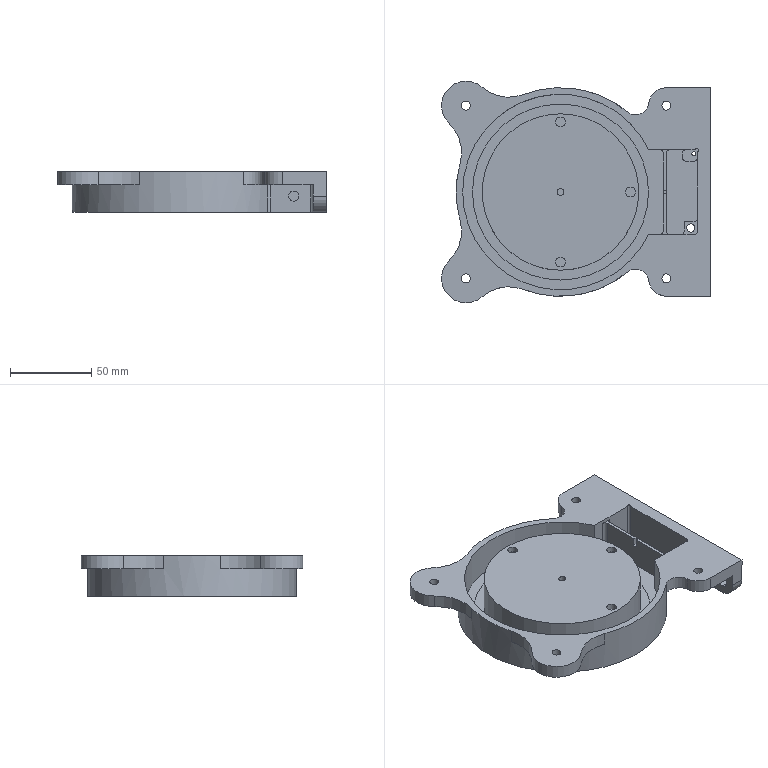NC program | NX | posted with a generic post | part box 165 x 136 x 25 mm
Lines 161 to 1182 of 5148:
(FLOOR_WALL_2 , TOOL : D10)
N308 T10 M6
N310 G54
N312 G17 G0 G90 X38.579 Y-66.122 S9500 M3
N314 G43 Z30. H10
N316 Z0.506
N318 G94 G1 Z-0.994 F1000.
N320 X37.578 Y-65.693
N322 G3 X36.585 Y-65.811 R1.
N324 G2 X27. Y-69. R16. F2500.
N326 G1 X13.1
N328 Y-35.1
N330 X32.479
N332 G3 X47.065 Y-52.494 R69.1
N334 G1 X47.053 Y-52.522
N336 G3 X42.885 Y-54.916 R3.
N338 G2 X36.585 Y-65.811 R16.
N340 G1 X33.59 Y-61.808
N342 G2 X27. Y-64. R11.
N344 G1 X18.1
N346 Y-40.1
N348 X29.688
N350 G3 X38.779 Y-51.559 R74.1
N352 X37.921 Y-54.317 R8.
N354 G2 X33.59 Y-61.808 R11.
N356 G1 X30.594 Y-57.804
N358 G2 X27. Y-59. R6.
N360 G1 X23.1
N362 Y-45.1
N364 X27.017
N366 G3 X33.101 Y-52.799 R79.1
N368 X32.957 Y-53.718 R13.
N370 G2 X30.594 Y-57.804 R6.
N372 G1 X27.899 Y-54.201
N374 G2 X27.6 Y-54.375 R1.5
N376 G1 Y-53.307
N378 G3 X28.15 Y-53.964 R83.6
N380 G2 X27.899 Y-54.201 R1.5
N382 G3 X27.505 Y-55.12 R1.
N384 G1 Z0.506
N386 G0 X38.579 Y-66.122 Z-0.488
N388 G1 Z-1.988 F1000.
N390 X37.578 Y-65.693
N392 G3 X36.585 Y-65.811 R1.
N394 G2 X27. Y-69. R16. F2500.
N396 G1 X13.1
N398 Y-35.1
N400 X32.479
N402 G3 X47.065 Y-52.494 R69.1
N404 G1 X47.053 Y-52.522
N406 G3 X42.885 Y-54.916 R3.
N408 G2 X36.585 Y-65.811 R16.
N410 G1 X33.59 Y-61.808
N412 G2 X27. Y-64. R11.
N414 G1 X18.1
N416 Y-40.1
N418 X29.688
N420 G3 X38.779 Y-51.559 R74.1
N422 X37.921 Y-54.317 R8.
N424 G2 X33.59 Y-61.808 R11.
N426 G1 X30.594 Y-57.804
N428 G2 X27. Y-59. R6.
N430 G1 X23.1
N432 Y-45.1
N434 X27.017
N436 G3 X33.101 Y-52.799 R79.1
N438 X32.957 Y-53.718 R13.
N440 G2 X30.594 Y-57.804 R6.
N442 G1 X27.899 Y-54.201
N444 G2 X27.6 Y-54.375 R1.5
N446 G1 Y-53.307
N448 G3 X28.15 Y-53.964 R83.6
N450 G2 X27.899 Y-54.201 R1.5
N452 G3 X27.505 Y-55.12 R1.
N454 G1 Z-0.488
N456 G0 X38.579 Y-66.122 Z-1.482
N458 G1 Z-2.982 F1000.
N460 X37.578 Y-65.693
N462 G3 X36.585 Y-65.811 R1.
N464 G2 X27. Y-69. R16. F2500.
N466 G1 X13.1
N468 Y-35.1
N470 X32.479
N472 G3 X47.065 Y-52.494 R69.1
N474 G1 X47.053 Y-52.522
N476 G3 X42.885 Y-54.916 R3.
N478 G2 X36.585 Y-65.811 R16.
N480 G1 X33.59 Y-61.808
N482 G2 X27. Y-64. R11.
N484 G1 X18.1
N486 Y-40.1
N488 X29.688
N490 G3 X38.779 Y-51.559 R74.1
N492 X37.921 Y-54.317 R8.
N494 G2 X33.59 Y-61.808 R11.
N496 G1 X30.594 Y-57.804
N498 G2 X27. Y-59. R6.
N500 G1 X23.1
N502 Y-45.1
N504 X27.017
N506 G3 X33.101 Y-52.799 R79.1
N508 X32.957 Y-53.718 R13.
N510 G2 X30.594 Y-57.804 R6.
N512 G1 X27.899 Y-54.201
N514 G2 X27.6 Y-54.375 R1.5
N516 G1 Y-53.307
N518 G3 X28.15 Y-53.964 R83.6
N520 G2 X27.899 Y-54.201 R1.5
N522 G3 X27.505 Y-55.12 R1.
N524 G1 Z-1.482
N526 G0 X38.579 Y-66.122 Z-2.476
N528 G1 Z-3.976 F1000.
N530 X37.578 Y-65.693
N532 G3 X36.585 Y-65.811 R1.
N534 G2 X27. Y-69. R16. F2500.
N536 G1 X13.1
N538 Y-35.1
N540 X32.479
N542 G3 X47.065 Y-52.494 R69.1
N544 G1 X47.053 Y-52.522
N546 G3 X42.885 Y-54.916 R3.
N548 G2 X36.585 Y-65.811 R16.
N550 G1 X33.59 Y-61.808
N552 G2 X27. Y-64. R11.
N554 G1 X18.1
N556 Y-40.1
N558 X29.688
N560 G3 X38.779 Y-51.559 R74.1
N562 X37.921 Y-54.317 R8.
N564 G2 X33.59 Y-61.808 R11.
N566 G1 X30.594 Y-57.804
N568 G2 X27. Y-59. R6.
N570 G1 X23.1
N572 Y-45.1
N574 X27.017
N576 G3 X33.101 Y-52.799 R79.1
N578 X32.957 Y-53.718 R13.
N580 G2 X30.594 Y-57.804 R6.
N582 G1 X27.899 Y-54.201
N584 G2 X27.6 Y-54.375 R1.5
N586 G1 Y-53.307
N588 G3 X28.15 Y-53.964 R83.6
N590 G2 X27.899 Y-54.201 R1.5
N592 G3 X27.505 Y-55.12 R1.
N594 G1 Z-2.476
N596 G0 X38.579 Y-66.122 Z-3.471
N598 G1 Z-4.971 F1000.
N600 X37.578 Y-65.693
N602 G3 X36.585 Y-65.811 R1.
N604 G2 X27. Y-69. R16. F2500.
N606 G1 X13.1
N608 Y-35.1
N610 X32.479
N612 G3 X47.065 Y-52.494 R69.1
N614 G1 X47.053 Y-52.522
N616 G3 X42.885 Y-54.916 R3.
N618 G2 X36.585 Y-65.811 R16.
N620 G1 X33.59 Y-61.808
N622 G2 X27. Y-64. R11.
N624 G1 X18.1
N626 Y-40.1
N628 X29.688
N630 G3 X38.779 Y-51.559 R74.1
N632 X37.921 Y-54.317 R8.
N634 G2 X33.59 Y-61.808 R11.
N636 G1 X30.594 Y-57.804
N638 G2 X27. Y-59. R6.
N640 G1 X23.1
N642 Y-45.1
N644 X27.017
N646 G3 X33.101 Y-52.799 R79.1
N648 X32.957 Y-53.718 R13.
N650 G2 X30.594 Y-57.804 R6.
N652 G1 X27.899 Y-54.201
N654 G2 X27.6 Y-54.375 R1.5
N656 G1 Y-53.307
N658 G3 X28.15 Y-53.964 R83.6
N660 G2 X27.899 Y-54.201 R1.5
N662 G3 X27.505 Y-55.12 R1.
N664 G1 Z-3.471
N666 G0 X38.579 Y-66.122 Z-4.465
N668 G1 Z-5.965 F1000.
N670 X37.578 Y-65.693
N672 G3 X36.585 Y-65.811 R1.
N674 G2 X27. Y-69. R16. F2500.
N676 G1 X13.1
N678 Y-35.1
N680 X32.479
N682 G3 X47.065 Y-52.494 R69.1
N684 G1 X47.053 Y-52.522
N686 G3 X42.885 Y-54.916 R3.
N688 G2 X36.585 Y-65.811 R16.
N690 G1 X33.59 Y-61.808
N692 G2 X27. Y-64. R11.
N694 G1 X18.1
N696 Y-40.1
N698 X29.688
N700 G3 X38.779 Y-51.559 R74.1
N702 X37.921 Y-54.317 R8.
N704 G2 X33.59 Y-61.808 R11.
N706 G1 X30.594 Y-57.804
N708 G2 X27. Y-59. R6.
N710 G1 X23.1
N712 Y-45.1
N714 X27.017
N716 G3 X33.101 Y-52.799 R79.1
N718 X32.957 Y-53.718 R13.
N720 G2 X30.594 Y-57.804 R6.
N722 G1 X27.899 Y-54.201
N724 G2 X27.6 Y-54.375 R1.5
N726 G1 Y-53.307
N728 G3 X28.15 Y-53.964 R83.6
N730 G2 X27.899 Y-54.201 R1.5
N732 G3 X27.505 Y-55.12 R1.
N734 G1 Z-4.465
N736 G0 X38.579 Y-66.122 Z-5.459
N738 G1 Z-6.959 F1000.
N740 X37.578 Y-65.693
N742 G3 X36.585 Y-65.811 R1.
N744 G2 X27. Y-69. R16. F2500.
N746 G1 X13.1
N748 Y-35.1
N750 X32.479
N752 G3 X47.065 Y-52.494 R69.1
N754 G1 X47.053 Y-52.522
N756 G3 X42.885 Y-54.916 R3.
N758 G2 X36.585 Y-65.811 R16.
N760 G1 X33.59 Y-61.808
N762 G2 X27. Y-64. R11.
N764 G1 X18.1
N766 Y-40.1
N768 X29.688
N770 G3 X38.779 Y-51.559 R74.1
N772 X37.921 Y-54.317 R8.
N774 G2 X33.59 Y-61.808 R11.
N776 G1 X30.594 Y-57.804
N778 G2 X27. Y-59. R6.
N780 G1 X23.1
N782 Y-45.1
N784 X27.017
N786 G3 X33.101 Y-52.799 R79.1
N788 X32.957 Y-53.718 R13.
N790 G2 X30.594 Y-57.804 R6.
N792 G1 X27.899 Y-54.201
N794 G2 X27.6 Y-54.375 R1.5
N796 G1 Y-53.307
N798 G3 X28.15 Y-53.964 R83.6
N800 G2 X27.899 Y-54.201 R1.5
N802 G3 X27.505 Y-55.12 R1.
N804 G1 Z-5.459
N806 G0 X38.579 Y-66.122 Z-6.453
N808 G1 Z-7.953 F1000.
N810 X37.578 Y-65.693
N812 G3 X36.585 Y-65.811 R1.
N814 G2 X27. Y-69. R16. F2500.
N816 G1 X13.1
N818 Y-35.1
N820 X32.479
N822 G3 X47.065 Y-52.494 R69.1
N824 G1 X47.053 Y-52.522
N826 G3 X42.885 Y-54.916 R3.
N828 G2 X36.585 Y-65.811 R16.
N830 G1 X33.59 Y-61.808
N832 G2 X27. Y-64. R11.
N834 G1 X18.1
N836 Y-40.1
N838 X29.688
N840 G3 X38.779 Y-51.559 R74.1
N842 X37.921 Y-54.317 R8.
N844 G2 X33.59 Y-61.808 R11.
N846 G1 X30.594 Y-57.804
N848 G2 X27. Y-59. R6.
N850 G1 X23.1
N852 Y-45.1
N854 X27.017
N856 G3 X33.101 Y-52.799 R79.1
N858 X32.957 Y-53.718 R13.
N860 G2 X30.594 Y-57.804 R6.
N862 G1 X27.899 Y-54.201
N864 G2 X27.6 Y-54.375 R1.5
N866 G1 Y-53.307
N868 G3 X28.15 Y-53.964 R83.6
N870 G2 X27.899 Y-54.201 R1.5
N872 G3 X27.505 Y-55.12 R1.
N874 G1 Z-6.453
N876 G0 X38.579 Y-66.122 Z-7.447
N878 G1 Z-8.947 F1000.
N880 X37.578 Y-65.693
N882 G3 X36.585 Y-65.811 R1.
N884 G2 X27. Y-69. R16. F2500.
N886 G1 X13.1
N888 Y-35.1
N890 X32.479
N892 G3 X47.065 Y-52.494 R69.1
N894 G1 X47.053 Y-52.522
N896 G3 X42.885 Y-54.916 R3.
N898 G2 X36.585 Y-65.811 R16.
N900 G1 X33.59 Y-61.808
N902 G2 X27. Y-64. R11.
N904 G1 X18.1
N906 Y-40.1
N908 X29.688
N910 G3 X38.779 Y-51.559 R74.1
N912 X37.921 Y-54.317 R8.
N914 G2 X33.59 Y-61.808 R11.
N916 G1 X30.594 Y-57.804
N918 G2 X27. Y-59. R6.
N920 G1 X23.1
N922 Y-45.1
N924 X27.017
N926 G3 X33.101 Y-52.799 R79.1
N928 X32.957 Y-53.718 R13.
N930 G2 X30.594 Y-57.804 R6.
N932 G1 X27.899 Y-54.201
N934 G2 X27.6 Y-54.375 R1.5
N936 G1 Y-53.307
N938 G3 X28.15 Y-53.964 R83.6
N940 G2 X27.899 Y-54.201 R1.5
N942 G3 X27.505 Y-55.12 R1.
N944 G1 Z-7.447
N946 G0 X38.579 Y-66.122 Z-8.441
N948 G1 Z-9.941 F1000.
N950 X37.578 Y-65.693
N952 G3 X36.585 Y-65.811 R1.
N954 G2 X27. Y-69. R16. F2500.
N956 G1 X13.1
N958 Y-35.1
N960 X32.479
N962 G3 X47.065 Y-52.494 R69.1
N964 G1 X47.053 Y-52.522
N966 G3 X42.885 Y-54.916 R3.
N968 G2 X36.585 Y-65.811 R16.
N970 G1 X33.59 Y-61.808
N972 G2 X27. Y-64. R11.
N974 G1 X18.1
N976 Y-40.1
N978 X29.688
N980 G3 X38.779 Y-51.559 R74.1
N982 X37.921 Y-54.317 R8.
N984 G2 X33.59 Y-61.808 R11.
N986 G1 X30.594 Y-57.804
N988 G2 X27. Y-59. R6.
N990 G1 X23.1
N992 Y-45.1
N994 X27.017
N996 G3 X33.101 Y-52.799 R79.1
N998 X32.957 Y-53.718 R13.
N1000 G2 X30.594 Y-57.804 R6.
N1002 G1 X27.899 Y-54.201
N1004 G2 X27.6 Y-54.375 R1.5
N1006 G1 Y-53.307
N1008 G3 X28.15 Y-53.964 R83.6
N1010 G2 X27.899 Y-54.201 R1.5
N1012 G3 X27.505 Y-55.12 R1.
N1014 G1 Z-8.441
N1016 G0 X38.579 Y-66.122 Z-9.435
N1018 G1 Z-10.935 F1000.
N1020 X37.578 Y-65.693
N1022 G3 X36.585 Y-65.811 R1.
N1024 G2 X27. Y-69. R16. F2500.
N1026 G1 X13.1
N1028 Y-35.1
N1030 X32.479
N1032 G3 X47.065 Y-52.494 R69.1
N1034 G1 X47.053 Y-52.522
N1036 G3 X42.885 Y-54.916 R3.
N1038 G2 X36.585 Y-65.811 R16.
N1040 G1 X33.59 Y-61.808
N1042 G2 X27. Y-64. R11.
N1044 G1 X18.1
N1046 Y-40.1
N1048 X29.688
N1050 G3 X38.779 Y-51.559 R74.1
N1052 X37.921 Y-54.317 R8.
N1054 G2 X33.59 Y-61.808 R11.
N1056 G1 X30.594 Y-57.804
N1058 G2 X27. Y-59. R6.
N1060 G1 X23.1
N1062 Y-45.1
N1064 X27.017
N1066 G3 X33.101 Y-52.799 R79.1
N1068 X32.957 Y-53.718 R13.
N1070 G2 X30.594 Y-57.804 R6.
N1072 G1 X27.899 Y-54.201
N1074 G2 X27.6 Y-54.375 R1.5
N1076 G1 Y-53.307
N1078 G3 X28.15 Y-53.964 R83.6
N1080 G2 X27.899 Y-54.201 R1.5
N1082 G3 X27.505 Y-55.12 R1.
N1084 G1 Z-9.435
N1086 G0 X38.579 Y-66.122 Z-10.429
N1088 G1 Z-11.929 F1000.
N1090 X37.578 Y-65.693
N1092 G3 X36.585 Y-65.811 R1.
N1094 G2 X27. Y-69. R16. F2500.
N1096 G1 X13.1
N1098 Y-35.1
N1100 X32.479
N1102 G3 X47.065 Y-52.494 R69.1
N1104 G1 X47.053 Y-52.522
N1106 G3 X42.885 Y-54.916 R3.
N1108 G2 X36.585 Y-65.811 R16.
N1110 G1 X33.59 Y-61.808
N1112 G2 X27. Y-64. R11.
N1114 G1 X18.1
N1116 Y-40.1
N1118 X29.688
N1120 G3 X38.779 Y-51.559 R74.1
N1122 X37.921 Y-54.317 R8.
N1124 G2 X33.59 Y-61.808 R11.
N1126 G1 X30.594 Y-57.804
N1128 G2 X27. Y-59. R6.
N1130 G1 X23.1
N1132 Y-45.1
N1134 X27.017
N1136 G3 X33.101 Y-52.799 R79.1
N1138 X32.957 Y-53.718 R13.
N1140 G2 X30.594 Y-57.804 R6.
N1142 G1 X27.899 Y-54.201
N1144 G2 X27.6 Y-54.375 R1.5
N1146 G1 Y-53.307
N1148 G3 X28.15 Y-53.964 R83.6
N1150 G2 X27.899 Y-54.201 R1.5
N1152 G3 X27.505 Y-55.12 R1.
N1154 G1 Z-10.429
N1156 G0 X38.579 Y-66.122 Z-11.424
N1158 G1 Z-12.924 F1000.
N1160 X37.578 Y-65.693
N1162 G3 X36.585 Y-65.811 R1.
N1164 G2 X27. Y-69. R16. F2500.
N1166 G1 X13.1
N1168 Y-35.1
N1170 X32.479
N1172 G3 X47.065 Y-52.494 R69.1
N1174 G1 X47.053 Y-52.522
N1176 G3 X42.885 Y-54.916 R3.
N1178 G2 X36.585 Y-65.811 R16.
N1180 G1 X33.59 Y-61.808
N1182 G2 X27. Y-64. R11.
N1184 G1 X18.1
N1186 Y-40.1
N1188 X29.688
N1190 G3 X38.779 Y-51.559 R74.1
N1192 X37.921 Y-54.317 R8.
N1194 G2 X33.59 Y-61.808 R11.
N1196 G1 X30.594 Y-57.804
N1198 G2 X27. Y-59. R6.
N1200 G1 X23.1
N1202 Y-45.1
N1204 X27.017
N1206 G3 X33.101 Y-52.799 R79.1
N1208 X32.957 Y-53.718 R13.
N1210 G2 X30.594 Y-57.804 R6.
N1212 G1 X27.899 Y-54.201
N1214 G2 X27.6 Y-54.375 R1.5
N1216 G1 Y-53.307
N1218 G3 X28.15 Y-53.964 R83.6
N1220 G2 X27.899 Y-54.201 R1.5
N1222 G3 X27.505 Y-55.12 R1.
N1224 G1 Z-11.424
N1226 G0 X38.579 Y-66.122 Z-12.418
N1228 G1 Z-13.918 F1000.
N1230 X37.578 Y-65.693
N1232 G3 X36.585 Y-65.811 R1.
N1234 G2 X27. Y-69. R16. F2500.
N1236 G1 X13.1
N1238 Y-35.1
N1240 X32.479
N1242 G3 X47.065 Y-52.494 R69.1
N1244 G1 X47.053 Y-52.522
N1246 G3 X42.885 Y-54.916 R3.
N1248 G2 X36.585 Y-65.811 R16.
N1250 G1 X33.59 Y-61.808
N1252 G2 X27. Y-64. R11.
N1254 G1 X18.1
N1256 Y-40.1
N1258 X29.688
N1260 G3 X38.779 Y-51.559 R74.1
N1262 X37.921 Y-54.317 R8.
N1264 G2 X33.59 Y-61.808 R11.
N1266 G1 X30.594 Y-57.804
N1268 G2 X27. Y-59. R6.
N1270 G1 X23.1
N1272 Y-45.1
N1274 X27.017
N1276 G3 X33.101 Y-52.799 R79.1
N1278 X32.957 Y-53.718 R13.
N1280 G2 X30.594 Y-57.804 R6.
N1282 G1 X27.899 Y-54.201
N1284 G2 X27.6 Y-54.375 R1.5
N1286 G1 Y-53.307
N1288 G3 X28.15 Y-53.964 R83.6
N1290 G2 X27.899 Y-54.201 R1.5
N1292 G3 X27.505 Y-55.12 R1.
N1294 G1 Z-12.418
N1296 G0 X38.579 Y-66.122 Z-13.412
N1298 G1 Z-14.912 F1000.
N1300 X37.578 Y-65.693
N1302 G3 X36.585 Y-65.811 R1.
N1304 G2 X27. Y-69. R16. F2500.
N1306 G1 X13.1
N1308 Y-35.1
N1310 X32.479
N1312 G3 X47.065 Y-52.494 R69.1
N1314 G1 X47.053 Y-52.522
N1316 G3 X42.885 Y-54.916 R3.
N1318 G2 X36.585 Y-65.811 R16.
N1320 G1 X33.59 Y-61.808
N1322 G2 X27. Y-64. R11.
N1324 G1 X18.1
N1326 Y-40.1
N1328 X29.688
N1330 G3 X38.779 Y-51.559 R74.1
N1332 X37.921 Y-54.317 R8.
N1334 G2 X33.59 Y-61.808 R11.
N1336 G1 X30.594 Y-57.804
N1338 G2 X27. Y-59. R6.
N1340 G1 X23.1
N1342 Y-45.1
N1344 X27.017
N1346 G3 X33.101 Y-52.799 R79.1
N1348 X32.957 Y-53.718 R13.
N1350 G2 X30.594 Y-57.804 R6.
N1352 G1 X27.899 Y-54.201
N1354 G2 X27.6 Y-54.375 R1.5
N1356 G1 Y-53.307
N1358 G3 X28.15 Y-53.964 R83.6
N1360 G2 X27.899 Y-54.201 R1.5
N1362 G3 X27.505 Y-55.12 R1.
N1364 G1 Z-13.412
N1366 G0 X38.579 Y-66.122 Z-14.406
N1368 G1 Z-15.906 F1000.
N1370 X37.578 Y-65.693
N1372 G3 X36.585 Y-65.811 R1.
N1374 G2 X27. Y-69. R16. F2500.
N1376 G1 X13.1
N1378 Y-35.1
N1380 X32.479
N1382 G3 X47.065 Y-52.494 R69.1
N1384 G1 X47.053 Y-52.522
N1386 G3 X42.885 Y-54.916 R3.
N1388 G2 X36.585 Y-65.811 R16.
N1390 G1 X33.59 Y-61.808
N1392 G2 X27. Y-64. R11.
N1394 G1 X18.1
N1396 Y-40.1
N1398 X29.688
N1400 G3 X38.779 Y-51.559 R74.1
N1402 X37.921 Y-54.317 R8.
N1404 G2 X33.59 Y-61.808 R11.
N1406 G1 X30.594 Y-57.804
N1408 G2 X27. Y-59. R6.
N1410 G1 X23.1
N1412 Y-45.1
N1414 X27.017
N1416 G3 X33.101 Y-52.799 R79.1
N1418 X32.957 Y-53.718 R13.
N1420 G2 X30.594 Y-57.804 R6.
N1422 G1 X27.899 Y-54.201
N1424 G2 X27.6 Y-54.375 R1.5
N1426 G1 Y-53.307
N1428 G3 X28.15 Y-53.964 R83.6
N1430 G2 X27.899 Y-54.201 R1.5
N1432 G3 X27.505 Y-55.12 R1.
N1434 G1 Z-14.406
N1436 G0 X38.579 Y-66.122 Z-15.4
N1438 G1 Z-16.9 F1000.
N1440 X37.578 Y-65.693
N1442 G3 X36.585 Y-65.811 R1.
N1444 G2 X27. Y-69. R16. F2500.
N1446 G1 X13.1
N1448 Y-35.1
N1450 X32.479
N1452 G3 X47.065 Y-52.494 R69.1
N1454 G1 X47.053 Y-52.522
N1456 G3 X42.885 Y-54.916 R3.
N1458 G2 X36.585 Y-65.811 R16.
N1460 G1 X33.59 Y-61.808
N1462 G2 X27. Y-64. R11.
N1464 G1 X18.1
N1466 Y-40.1
N1468 X29.688
N1470 G3 X38.779 Y-51.559 R74.1
N1472 X37.921 Y-54.317 R8.
N1474 G2 X33.59 Y-61.808 R11.
N1476 G1 X30.594 Y-57.804
N1478 G2 X27. Y-59. R6.
N1480 G1 X23.1
N1482 Y-45.1
N1484 X27.017
N1486 G3 X33.101 Y-52.799 R79.1
N1488 X32.957 Y-53.718 R13.
N1490 G2 X30.594 Y-57.804 R6.
N1492 G1 X27.899 Y-54.201
N1494 G2 X27.6 Y-54.375 R1.5
N1496 G1 Y-53.307
N1498 G3 X28.15 Y-53.964 R83.6
N1500 G2 X27.899 Y-54.201 R1.5
N1502 G3 X27.505 Y-55.12 R1.
N1504 G1 Z-15.4
N1506 G0 Z30.
N1508 X36.32 Y67.812
N1510 Z0.506
N1512 G1 Z-0.994 F1000.
N1514 X36.191 Y66.73
N1516 G3 X36.585 Y65.811 R1.
N1518 G2 X42.885 Y54.916 R16. F2500.
N1520 G3 X47.053 Y52.522 R3.
N1522 G1 X47.065 Y52.494
N1524 G3 X32.479 Y35.1 R69.1
N1526 G1 X13.1
N1528 Y69.
N1530 X27.
N1532 G2 X36.585 Y65.811 R16.
N1534 G1 X33.59 Y61.808
N1536 G2 X37.921 Y54.317 R11.
N1538 G3 X38.779 Y51.559 R8.
N1540 X29.688 Y40.1 R74.1
N1542 G1 X18.1
N1544 Y64.
N1546 X27.
N1548 G2 X33.59 Y61.808 R11.
N1550 G1 X30.594 Y57.804
N1552 G2 X32.957 Y53.719 R6.
N1554 G3 X33.101 Y52.799 R13.
N1556 X27.017 Y45.1 R79.1
N1558 G1 X23.1
N1560 Y59.
N1562 X27.
N1564 G2 X30.594 Y57.804 R6.
N1566 G1 X27.899 Y54.201
N1568 G2 X28.15 Y53.964 R1.5
N1570 G3 X27.6 Y53.307 R83.6
N1572 G1 Y54.375
N1574 G2 X27.899 Y54.201 R1.5
N1576 G3 X28.892 Y54.083 R1.
N1578 G1 Z0.506
N1580 G0 X36.32 Y67.812 Z-0.488
N1582 G1 Z-1.988 F1000.
N1584 X36.191 Y66.73
N1586 G3 X36.585 Y65.811 R1.
N1588 G2 X42.885 Y54.916 R16. F2500.
N1590 G3 X47.053 Y52.522 R3.
N1592 G1 X47.065 Y52.494
N1594 G3 X32.479 Y35.1 R69.1
N1596 G1 X13.1
N1598 Y69.
N1600 X27.
N1602 G2 X36.585 Y65.811 R16.
N1604 G1 X33.59 Y61.808
N1606 G2 X37.921 Y54.317 R11.
N1608 G3 X38.779 Y51.559 R8.
N1610 X29.688 Y40.1 R74.1
N1612 G1 X18.1
N1614 Y64.
N1616 X27.
N1618 G2 X33.59 Y61.808 R11.
N1620 G1 X30.594 Y57.804
N1622 G2 X32.957 Y53.719 R6.
N1624 G3 X33.101 Y52.799 R13.
N1626 X27.017 Y45.1 R79.1
N1628 G1 X23.1
N1630 Y59.
N1632 X27.
N1634 G2 X30.594 Y57.804 R6.
N1636 G1 X27.899 Y54.201
N1638 G2 X28.15 Y53.964 R1.5
N1640 G3 X27.6 Y53.307 R83.6
N1642 G1 Y54.375
N1644 G2 X27.899 Y54.201 R1.5
N1646 G3 X28.892 Y54.083 R1.
N1648 G1 Z-0.488
N1650 G0 X36.32 Y67.812 Z-1.482
N1652 G1 Z-2.982 F1000.
N1654 X36.191 Y66.73
N1656 G3 X36.585 Y65.811 R1.
N1658 G2 X42.885 Y54.916 R16. F2500.
N1660 G3 X47.053 Y52.522 R3.
N1662 G1 X47.065 Y52.494
N1664 G3 X32.479 Y35.1 R69.1
N1666 G1 X13.1
N1668 Y69.
N1670 X27.
N1672 G2 X36.585 Y65.811 R16.
N1674 G1 X33.59 Y61.808
N1676 G2 X37.921 Y54.317 R11.
N1678 G3 X38.779 Y51.559 R8.
N1680 X29.688 Y40.1 R74.1
N1682 G1 X18.1
N1684 Y64.
N1686 X27.
N1688 G2 X33.59 Y61.808 R11.
N1690 G1 X30.594 Y57.804
N1692 G2 X32.957 Y53.719 R6.
N1694 G3 X33.101 Y52.799 R13.
N1696 X27.017 Y45.1 R79.1
N1698 G1 X23.1
N1700 Y59.
N1702 X27.
N1704 G2 X30.594 Y57.804 R6.
N1706 G1 X27.899 Y54.201
N1708 G2 X28.15 Y53.964 R1.5
N1710 G3 X27.6 Y53.307 R83.6
N1712 G1 Y54.375
N1714 G2 X27.899 Y54.201 R1.5
N1716 G3 X28.892 Y54.083 R1.
N1718 G1 Z-1.482
N1720 G0 X36.32 Y67.812 Z-2.476
N1722 G1 Z-3.976 F1000.
N1724 X36.191 Y66.73
N1726 G3 X36.585 Y65.811 R1.
N1728 G2 X42.885 Y54.916 R16. F2500.
N1730 G3 X47.053 Y52.522 R3.
N1732 G1 X47.065 Y52.494
N1734 G3 X32.479 Y35.1 R69.1
N1736 G1 X13.1
N1738 Y69.
N1740 X27.
N1742 G2 X36.585 Y65.811 R16.
N1744 G1 X33.59 Y61.808
N1746 G2 X37.921 Y54.317 R11.
N1748 G3 X38.779 Y51.559 R8.
N1750 X29.688 Y40.1 R74.1
N1752 G1 X18.1
N1754 Y64.
N1756 X27.
N1758 G2 X33.59 Y61.808 R11.
N1760 G1 X30.594 Y57.804
N1762 G2 X32.957 Y53.719 R6.
N1764 G3 X33.101 Y52.799 R13.
N1766 X27.017 Y45.1 R79.1
N1768 G1 X23.1
N1770 Y59.
N1772 X27.
N1774 G2 X30.594 Y57.804 R6.
N1776 G1 X27.899 Y54.201
N1778 G2 X28.15 Y53.964 R1.5
N1780 G3 X27.6 Y53.307 R83.6
N1782 G1 Y54.375
N1784 G2 X27.899 Y54.201 R1.5
N1786 G3 X28.892 Y54.083 R1.
N1788 G1 Z-2.476
N1790 G0 X36.32 Y67.812 Z-3.471
N1792 G1 Z-4.971 F1000.
N1794 X36.191 Y66.73
N1796 G3 X36.585 Y65.811 R1.
N1798 G2 X42.885 Y54.916 R16. F2500.
N1800 G3 X47.053 Y52.522 R3.
N1802 G1 X47.065 Y52.494
N1804 G3 X32.479 Y35.1 R69.1
N1806 G1 X13.1
N1808 Y69.
N1810 X27.
N1812 G2 X36.585 Y65.811 R16.
N1814 G1 X33.59 Y61.808
N1816 G2 X37.921 Y54.317 R11.
N1818 G3 X38.779 Y51.559 R8.
N1820 X29.688 Y40.1 R74.1
N1822 G1 X18.1
N1824 Y64.
N1826 X27.
N1828 G2 X33.59 Y61.808 R11.
N1830 G1 X30.594 Y57.804
N1832 G2 X32.957 Y53.719 R6.
N1834 G3 X33.101 Y52.799 R13.
N1836 X27.017 Y45.1 R79.1
N1838 G1 X23.1
N1840 Y59.
N1842 X27.
N1844 G2 X30.594 Y57.804 R6.
N1846 G1 X27.899 Y54.201
N1848 G2 X28.15 Y53.964 R1.5
N1850 G3 X27.6 Y53.307 R83.6
N1852 G1 Y54.375
N1854 G2 X27.899 Y54.201 R1.5
N1856 G3 X28.892 Y54.083 R1.
N1858 G1 Z-3.471
N1860 G0 X36.32 Y67.812 Z-4.465
N1862 G1 Z-5.965 F1000.
N1864 X36.191 Y66.73
N1866 G3 X36.585 Y65.811 R1.
N1868 G2 X42.885 Y54.916 R16. F2500.
N1870 G3 X47.053 Y52.522 R3.
N1872 G1 X47.065 Y52.494
N1874 G3 X32.479 Y35.1 R69.1
N1876 G1 X13.1
N1878 Y69.
N1880 X27.
N1882 G2 X36.585 Y65.811 R16.
N1884 G1 X33.59 Y61.808
N1886 G2 X37.921 Y54.317 R11.
N1888 G3 X38.779 Y51.559 R8.
N1890 X29.688 Y40.1 R74.1
N1892 G1 X18.1
N1894 Y64.
N1896 X27.
N1898 G2 X33.59 Y61.808 R11.
N1900 G1 X30.594 Y57.804
N1902 G2 X32.957 Y53.719 R6.
N1904 G3 X33.101 Y52.799 R13.
N1906 X27.017 Y45.1 R79.1
N1908 G1 X23.1
N1910 Y59.
N1912 X27.
N1914 G2 X30.594 Y57.804 R6.
N1916 G1 X27.899 Y54.201
N1918 G2 X28.15 Y53.964 R1.5
N1920 G3 X27.6 Y53.307 R83.6
N1922 G1 Y54.375
N1924 G2 X27.899 Y54.201 R1.5
N1926 G3 X28.892 Y54.083 R1.
N1928 G1 Z-4.465
N1930 G0 X36.32 Y67.812 Z-5.459
N1932 G1 Z-6.959 F1000.
N1934 X36.191 Y66.73
N1936 G3 X36.585 Y65.811 R1.
N1938 G2 X42.885 Y54.916 R16. F2500.
N1940 G3 X47.053 Y52.522 R3.
N1942 G1 X47.065 Y52.494
N1944 G3 X32.479 Y35.1 R69.1
N1946 G1 X13.1
N1948 Y69.
N1950 X27.
N1952 G2 X36.585 Y65.811 R16.
N1954 G1 X33.59 Y61.808
N1956 G2 X37.921 Y54.317 R11.
N1958 G3 X38.779 Y51.559 R8.
N1960 X29.688 Y40.1 R74.1
N1962 G1 X18.1
N1964 Y64.
N1966 X27.
N1968 G2 X33.59 Y61.808 R11.
N1970 G1 X30.594 Y57.804
N1972 G2 X32.957 Y53.719 R6.
N1974 G3 X33.101 Y52.799 R13.
N1976 X27.017 Y45.1 R79.1
N1978 G1 X23.1
N1980 Y59.
N1982 X27.
N1984 G2 X30.594 Y57.804 R6.
N1986 G1 X27.899 Y54.201
N1988 G2 X28.15 Y53.964 R1.5
N1990 G3 X27.6 Y53.307 R83.6
N1992 G1 Y54.375
N1994 G2 X27.899 Y54.201 R1.5
N1996 G3 X28.892 Y54.083 R1.
N1998 G1 Z-5.459
N2000 G0 X36.32 Y67.812 Z-6.453
N2002 G1 Z-7.953 F1000.
N2004 X36.191 Y66.73
N2006 G3 X36.585 Y65.811 R1.
N2008 G2 X42.885 Y54.916 R16. F2500.
N2010 G3 X47.053 Y52.522 R3.
N2012 G1 X47.065 Y52.494
N2014 G3 X32.479 Y35.1 R69.1
N2016 G1 X13.1
N2018 Y69.
N2020 X27.
N2022 G2 X36.585 Y65.811 R16.
N2024 G1 X33.59 Y61.808
N2026 G2 X37.921 Y54.317 R11.
N2028 G3 X38.779 Y51.559 R8.
N2030 X29.688 Y40.1 R74.1
N2032 G1 X18.1
N2034 Y64.
N2036 X27.
N2038 G2 X33.59 Y61.808 R11.
N2040 G1 X30.594 Y57.804
N2042 G2 X32.957 Y53.719 R6.
N2044 G3 X33.101 Y52.799 R13.
N2046 X27.017 Y45.1 R79.1
N2048 G1 X23.1
N2050 Y59.
N2052 X27.
N2054 G2 X30.594 Y57.804 R6.
N2056 G1 X27.899 Y54.201
N2058 G2 X28.15 Y53.964 R1.5
N2060 G3 X27.6 Y53.307 R83.6
N2062 G1 Y54.375
N2064 G2 X27.899 Y54.201 R1.5
N2066 G3 X28.892 Y54.083 R1.
N2068 G1 Z-6.453
N2070 G0 X36.32 Y67.812 Z-7.447
N2072 G1 Z-8.947 F1000.
N2074 X36.191 Y66.73
N2076 G3 X36.585 Y65.811 R1.
N2078 G2 X42.885 Y54.916 R16. F2500.
N2080 G3 X47.053 Y52.522 R3.
N2082 G1 X47.065 Y52.494
N2084 G3 X32.479 Y35.1 R69.1
N2086 G1 X13.1
N2088 Y69.
N2090 X27.
N2092 G2 X36.585 Y65.811 R16.
N2094 G1 X33.59 Y61.808
N2096 G2 X37.921 Y54.317 R11.
N2098 G3 X38.779 Y51.559 R8.
N2100 X29.688 Y40.1 R74.1
N2102 G1 X18.1
N2104 Y64.
N2106 X27.
N2108 G2 X33.59 Y61.808 R11.
N2110 G1 X30.594 Y57.804
N2112 G2 X32.957 Y53.719 R6.
N2114 G3 X33.101 Y52.799 R13.
N2116 X27.017 Y45.1 R79.1
N2118 G1 X23.1
N2120 Y59.
N2122 X27.
N2124 G2 X30.594 Y57.804 R6.
N2126 G1 X27.899 Y54.201
N2128 G2 X28.15 Y53.964 R1.5
N2130 G3 X27.6 Y53.307 R83.6
N2132 G1 Y54.375
N2134 G2 X27.899 Y54.201 R1.5
N2136 G3 X28.892 Y54.083 R1.
N2138 G1 Z-7.447
N2140 G0 X36.32 Y67.812 Z-8.441
N2142 G1 Z-9.941 F1000.
N2144 X36.191 Y66.73
N2146 G3 X36.585 Y65.811 R1.
N2148 G2 X42.885 Y54.916 R16. F2500.
N2150 G3 X47.053 Y52.522 R3.
N2152 G1 X47.065 Y52.494
N2154 G3 X32.479 Y35.1 R69.1
N2156 G1 X13.1
N2158 Y69.
N2160 X27.
N2162 G2 X36.585 Y65.811 R16.
N2164 G1 X33.59 Y61.808
N2166 G2 X37.921 Y54.317 R11.
N2168 G3 X38.779 Y51.559 R8.
N2170 X29.688 Y40.1 R74.1
N2172 G1 X18.1
N2174 Y64.
N2176 X27.
N2178 G2 X33.59 Y61.808 R11.
N2180 G1 X30.594 Y57.804
N2182 G2 X32.957 Y53.719 R6.
N2184 G3 X33.101 Y52.799 R13.
N2186 X27.017 Y45.1 R79.1
N2188 G1 X23.1
N2190 Y59.
N2192 X27.
N2194 G2 X30.594 Y57.804 R6.
N2196 G1 X27.899 Y54.201
N2198 G2 X28.15 Y53.964 R1.5
N2200 G3 X27.6 Y53.307 R83.6
N2202 G1 Y54.375
N2204 G2 X27.899 Y54.201 R1.5
N2206 G3 X28.892 Y54.083 R1.
N2208 G1 Z-8.441
N2210 G0 X36.32 Y67.812 Z-9.435
N2212 G1 Z-10.935 F1000.
N2214 X36.191 Y66.73
N2216 G3 X36.585 Y65.811 R1.
N2218 G2 X42.885 Y54.916 R16. F2500.
N2220 G3 X47.053 Y52.522 R3.
N2222 G1 X47.065 Y52.494
N2224 G3 X32.479 Y35.1 R69.1
N2226 G1 X13.1
N2228 Y69.
N2230 X27.
N2232 G2 X36.585 Y65.811 R16.
N2234 G1 X33.59 Y61.808
N2236 G2 X37.921 Y54.317 R11.
N2238 G3 X38.779 Y51.559 R8.
N2240 X29.688 Y40.1 R74.1
N2242 G1 X18.1
N2244 Y64.
N2246 X27.
N2248 G2 X33.59 Y61.808 R11.
N2250 G1 X30.594 Y57.804
N2252 G2 X32.957 Y53.719 R6.
N2254 G3 X33.101 Y52.799 R13.
N2256 X27.017 Y45.1 R79.1
N2258 G1 X23.1
N2260 Y59.
N2262 X27.
N2264 G2 X30.594 Y57.804 R6.
N2266 G1 X27.899 Y54.201
N2268 G2 X28.15 Y53.964 R1.5
N2270 G3 X27.6 Y53.307 R83.6
N2272 G1 Y54.375
N2274 G2 X27.899 Y54.201 R1.5
N2276 G3 X28.892 Y54.083 R1.
N2278 G1 Z-9.435
N2280 G0 X36.32 Y67.812 Z-10.429
N2282 G1 Z-11.929 F1000.
N2284 X36.191 Y66.73
N2286 G3 X36.585 Y65.811 R1.
N2288 G2 X42.885 Y54.916 R16. F2500.
N2290 G3 X47.053 Y52.522 R3.
N2292 G1 X47.065 Y52.494
N2294 G3 X32.479 Y35.1 R69.1
N2296 G1 X13.1
N2298 Y69.
N2300 X27.
N2302 G2 X36.585 Y65.811 R16.
N2304 G1 X33.59 Y61.808
N2306 G2 X37.921 Y54.317 R11.
N2308 G3 X38.779 Y51.559 R8.
N2310 X29.688 Y40.1 R74.1
N2312 G1 X18.1
N2314 Y64.
N2316 X27.
N2318 G2 X33.59 Y61.808 R11.
N2320 G1 X30.594 Y57.804
N2322 G2 X32.957 Y53.719 R6.
N2324 G3 X33.101 Y52.799 R13.
N2326 X27.017 Y45.1 R79.1
N2328 G1 X23.1
N2330 Y59.
N2332 X27.
N2334 G2 X30.594 Y57.804 R6.
N2336 G1 X27.899 Y54.201
N2338 G2 X28.15 Y53.964 R1.5
N2340 G3 X27.6 Y53.307 R83.6
N2342 G1 Y54.375
N2344 G2 X27.899 Y54.201 R1.5